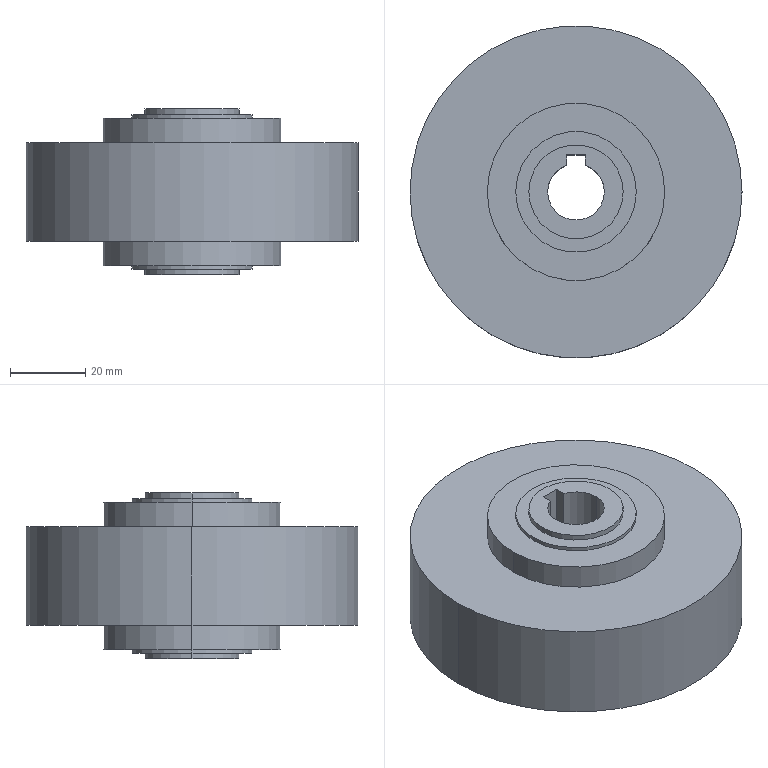Part | STEP file | Mirror ZX3YN | 1 solid | 40 faces | box 88 x 88 x 44 mm | volume 175155 mm3 | cylinder 23 | plane 11 | cone 6 | commonest cylinder face diameters 3.3 x6 25 x4 32 x4 47 x4 15 x3 88 x2
STEP:
#1=CARTESIAN_POINT('',(-35.466,-18.571,-1.5));
#2=VERTEX_POINT('',#1);
#3=CARTESIAN_POINT('',(-33.816,-21.429,-1.5));
#4=VERTEX_POINT('',#3);
#5=CARTESIAN_POINT('',(-34.641,-20.,-1.5));
#6=DIRECTION('',(0.,0.,1.));
#7=DIRECTION('',(-0.5,0.866,0.));
#8=AXIS2_PLACEMENT_3D('',#5,#6,#7);
#9=CIRCLE('',#8,1.65);
#10=EDGE_CURVE('',#2,#4,#9,.T.);
#11=ORIENTED_EDGE('',*,*,#10,.T.);
#12=CARTESIAN_POINT('',(-33.816,-21.429,-13.));
#13=VERTEX_POINT('',#12);
#14=CARTESIAN_POINT('',(-33.816,-21.429,-13.));
#15=DIRECTION('',(0.,0.,-1.));
#16=VECTOR('',#15,1000.);
#17=LINE('',#14,#16);
#18=EDGE_CURVE('',#4,#13,#17,.T.);
#19=ORIENTED_EDGE('',*,*,#18,.T.);
#20=CARTESIAN_POINT('',(-35.466,-18.571,-13.));
#21=VERTEX_POINT('',#20);
#22=CARTESIAN_POINT('',(-34.641,-20.,-13.));
#23=DIRECTION('',(0.,0.,1.));
#24=DIRECTION('',(-0.5,0.866,0.));
#25=AXIS2_PLACEMENT_3D('',#22,#23,#24);
#26=CIRCLE('',#25,1.65);
#27=EDGE_CURVE('',#21,#13,#26,.T.);
#28=ORIENTED_EDGE('',*,*,#27,.F.);
#29=CARTESIAN_POINT('',(-35.466,-18.571,-13.));
#30=DIRECTION('',(0.,0.,-1.));
#31=VECTOR('',#30,1000.);
#32=LINE('',#29,#31);
#33=EDGE_CURVE('',#2,#21,#32,.T.);
#34=ORIENTED_EDGE('',*,*,#33,.F.);
#35=EDGE_LOOP('',(#11,#19,#28,#34));
#36=FACE_OUTER_BOUND('',#35,.T.);
#37=CARTESIAN_POINT('',(-34.641,-20.,-13.));
#38=DIRECTION('',(0.,0.,-1.));
#39=DIRECTION('',(-0.5,0.866,0.));
#40=AXIS2_PLACEMENT_3D('',#37,#38,#39);
#41=CYLINDRICAL_SURFACE('',#40,1.65);
#42=ADVANCED_FACE('',(#36),#41,.F.);
#43=CARTESIAN_POINT('',(-34.641,-20.,-0.5086));
#44=VERTEX_POINT('',#43);
#45=CARTESIAN_POINT('',(-35.466,-18.571,-1.5));
#46=DIRECTION('',(-0.4286,0.7423,-0.515));
#47=VECTOR('',#46,1000.);
#48=LINE('',#45,#47);
#49=EDGE_CURVE('',#44,#2,#48,.T.);
#50=ORIENTED_EDGE('',*,*,#49,.F.);
#51=CARTESIAN_POINT('',(-33.816,-21.429,-1.5));
#52=DIRECTION('',(0.4286,-0.7423,-0.515));
#53=VECTOR('',#52,1000.);
#54=LINE('',#51,#53);
#55=EDGE_CURVE('',#44,#4,#54,.T.);
#56=ORIENTED_EDGE('',*,*,#55,.T.);
#57=ORIENTED_EDGE('',*,*,#10,.F.);
#58=EDGE_LOOP('',(#50,#56,#57));
#59=FACE_OUTER_BOUND('',#58,.T.);
#60=CARTESIAN_POINT('',(-34.641,-20.,-1.5));
#61=DIRECTION('',(0.,0.,-1.));
#62=DIRECTION('',(-0.5,0.866,0.));
#63=AXIS2_PLACEMENT_3D('',#60,#61,#62);
#64=CONICAL_SURFACE('',#63,1.65,1.03);
#65=ADVANCED_FACE('',(#59),#64,.F.);
#66=CARTESIAN_POINT('',(33.816,-21.429,-1.5));
#67=VERTEX_POINT('',#66);
#68=CARTESIAN_POINT('',(35.466,-18.571,-1.5));
#69=VERTEX_POINT('',#68);
#70=CARTESIAN_POINT('',(34.641,-20.,-1.5));
#71=DIRECTION('',(0.,0.,1.));
#72=DIRECTION('',(-0.5,-0.866,0.));
#73=AXIS2_PLACEMENT_3D('',#70,#71,#72);
#74=CIRCLE('',#73,1.65);
#75=EDGE_CURVE('',#67,#69,#74,.T.);
#76=ORIENTED_EDGE('',*,*,#75,.T.);
#77=CARTESIAN_POINT('',(35.466,-18.571,-13.));
#78=VERTEX_POINT('',#77);
#79=CARTESIAN_POINT('',(35.466,-18.571,-13.));
#80=DIRECTION('',(0.,0.,-1.));
#81=VECTOR('',#80,1000.);
#82=LINE('',#79,#81);
#83=EDGE_CURVE('',#69,#78,#82,.T.);
#84=ORIENTED_EDGE('',*,*,#83,.T.);
#85=CARTESIAN_POINT('',(33.816,-21.429,-13.));
#86=VERTEX_POINT('',#85);
#87=CARTESIAN_POINT('',(34.641,-20.,-13.));
#88=DIRECTION('',(0.,0.,1.));
#89=DIRECTION('',(-0.5,-0.866,0.));
#90=AXIS2_PLACEMENT_3D('',#87,#88,#89);
#91=CIRCLE('',#90,1.65);
#92=EDGE_CURVE('',#86,#78,#91,.T.);
#93=ORIENTED_EDGE('',*,*,#92,.F.);
#94=CARTESIAN_POINT('',(33.816,-21.429,-13.));
#95=DIRECTION('',(0.,0.,-1.));
#96=VECTOR('',#95,1000.);
#97=LINE('',#94,#96);
#98=EDGE_CURVE('',#67,#86,#97,.T.);
#99=ORIENTED_EDGE('',*,*,#98,.F.);
#100=EDGE_LOOP('',(#76,#84,#93,#99));
#101=FACE_OUTER_BOUND('',#100,.T.);
#102=CARTESIAN_POINT('',(34.641,-20.,-13.));
#103=DIRECTION('',(0.,0.,-1.));
#104=DIRECTION('',(-0.5,-0.866,0.));
#105=AXIS2_PLACEMENT_3D('',#102,#103,#104);
#106=CYLINDRICAL_SURFACE('',#105,1.65);
#107=ADVANCED_FACE('',(#101),#106,.F.);
#108=CARTESIAN_POINT('',(34.641,-20.,-0.5086));
#109=VERTEX_POINT('',#108);
#110=CARTESIAN_POINT('',(33.816,-21.429,-1.5));
#111=DIRECTION('',(-0.4286,-0.7423,-0.515));
#112=VECTOR('',#111,1000.);
#113=LINE('',#110,#112);
#114=EDGE_CURVE('',#109,#67,#113,.T.);
#115=ORIENTED_EDGE('',*,*,#114,.F.);
#116=CARTESIAN_POINT('',(35.466,-18.571,-1.5));
#117=DIRECTION('',(0.4286,0.7423,-0.515));
#118=VECTOR('',#117,1000.);
#119=LINE('',#116,#118);
#120=EDGE_CURVE('',#109,#69,#119,.T.);
#121=ORIENTED_EDGE('',*,*,#120,.T.);
#122=ORIENTED_EDGE('',*,*,#75,.F.);
#123=EDGE_LOOP('',(#115,#121,#122));
#124=FACE_OUTER_BOUND('',#123,.T.);
#125=CARTESIAN_POINT('',(34.641,-20.,-1.5));
#126=DIRECTION('',(0.,0.,-1.));
#127=DIRECTION('',(-0.5,-0.866,0.));
#128=AXIS2_PLACEMENT_3D('',#125,#126,#127);
#129=CONICAL_SURFACE('',#128,1.65,1.03);
#130=ADVANCED_FACE('',(#124),#129,.F.);
#131=CARTESIAN_POINT('',(1.65,40.,-1.5));
#132=VERTEX_POINT('',#131);
#133=CARTESIAN_POINT('',(-1.65,40.,-1.5));
#134=VERTEX_POINT('',#133);
#135=CARTESIAN_POINT('',(0.,40.,-1.5));
#136=DIRECTION('',(0.,0.,1.));
#137=DIRECTION('',(1.,0.,0.));
#138=AXIS2_PLACEMENT_3D('',#135,#136,#137);
#139=CIRCLE('',#138,1.65);
#140=EDGE_CURVE('',#132,#134,#139,.T.);
#141=ORIENTED_EDGE('',*,*,#140,.T.);
#142=CARTESIAN_POINT('',(-1.65,40.,-13.));
#143=VERTEX_POINT('',#142);
#144=CARTESIAN_POINT('',(-1.65,40.,-13.));
#145=DIRECTION('',(0.,0.,-1.));
#146=VECTOR('',#145,1000.);
#147=LINE('',#144,#146);
#148=EDGE_CURVE('',#134,#143,#147,.T.);
#149=ORIENTED_EDGE('',*,*,#148,.T.);
#150=CARTESIAN_POINT('',(1.65,40.,-13.));
#151=VERTEX_POINT('',#150);
#152=CARTESIAN_POINT('',(0.,40.,-13.));
#153=DIRECTION('',(0.,0.,1.));
#154=DIRECTION('',(1.,0.,0.));
#155=AXIS2_PLACEMENT_3D('',#152,#153,#154);
#156=CIRCLE('',#155,1.65);
#157=EDGE_CURVE('',#151,#143,#156,.T.);
#158=ORIENTED_EDGE('',*,*,#157,.F.);
#159=CARTESIAN_POINT('',(1.65,40.,-13.));
#160=DIRECTION('',(0.,0.,-1.));
#161=VECTOR('',#160,1000.);
#162=LINE('',#159,#161);
#163=EDGE_CURVE('',#132,#151,#162,.T.);
#164=ORIENTED_EDGE('',*,*,#163,.F.);
#165=EDGE_LOOP('',(#141,#149,#158,#164));
#166=FACE_OUTER_BOUND('',#165,.T.);
#167=CARTESIAN_POINT('',(0.,40.,-13.));
#168=DIRECTION('',(0.,0.,-1.));
#169=DIRECTION('',(1.,0.,0.));
#170=AXIS2_PLACEMENT_3D('',#167,#168,#169);
#171=CYLINDRICAL_SURFACE('',#170,1.65);
#172=ADVANCED_FACE('',(#166),#171,.F.);
#173=CARTESIAN_POINT('',(0.,40.,-0.5086));
#174=VERTEX_POINT('',#173);
#175=CARTESIAN_POINT('',(1.65,40.,-1.5));
#176=DIRECTION('',(0.8572,0.,-0.515));
#177=VECTOR('',#176,1000.);
#178=LINE('',#175,#177);
#179=EDGE_CURVE('',#174,#132,#178,.T.);
#180=ORIENTED_EDGE('',*,*,#179,.F.);
#181=CARTESIAN_POINT('',(-1.65,40.,-1.5));
#182=DIRECTION('',(-0.8572,0.,-0.515));
#183=VECTOR('',#182,1000.);
#184=LINE('',#181,#183);
#185=EDGE_CURVE('',#174,#134,#184,.T.);
#186=ORIENTED_EDGE('',*,*,#185,.T.);
#187=ORIENTED_EDGE('',*,*,#140,.F.);
#188=EDGE_LOOP('',(#180,#186,#187));
#189=FACE_OUTER_BOUND('',#188,.T.);
#190=CARTESIAN_POINT('',(0.,40.,-1.5));
#191=DIRECTION('',(0.,0.,-1.));
#192=DIRECTION('',(1.,0.,0.));
#193=AXIS2_PLACEMENT_3D('',#190,#191,#192);
#194=CONICAL_SURFACE('',#193,1.65,1.03);
#195=ADVANCED_FACE('',(#189),#194,.F.);
#196=CARTESIAN_POINT('',(-2.5,7.071,22.));
#197=VERTEX_POINT('',#196);
#198=CARTESIAN_POINT('',(-7.5,0.,22.));
#199=VERTEX_POINT('',#198);
#200=CARTESIAN_POINT('',(0.,0.,22.));
#201=DIRECTION('',(0.,0.,1.));
#202=DIRECTION('',(1.,0.,0.));
#203=AXIS2_PLACEMENT_3D('',#200,#201,#202);
#204=CIRCLE('',#203,7.5);
#205=EDGE_CURVE('',#197,#199,#204,.T.);
#206=ORIENTED_EDGE('',*,*,#205,.T.);
#207=CARTESIAN_POINT('',(-7.5,0.,-22.));
#208=VERTEX_POINT('',#207);
#209=CARTESIAN_POINT('',(-7.5,0.,22.));
#210=DIRECTION('',(0.,0.,-1.));
#211=VECTOR('',#210,1000.);
#212=LINE('',#209,#211);
#213=EDGE_CURVE('',#199,#208,#212,.T.);
#214=ORIENTED_EDGE('',*,*,#213,.T.);
#215=CARTESIAN_POINT('',(-2.5,7.071,-22.));
#216=VERTEX_POINT('',#215);
#217=CARTESIAN_POINT('',(0.,0.,-22.));
#218=DIRECTION('',(0.,0.,1.));
#219=DIRECTION('',(1.,0.,0.));
#220=AXIS2_PLACEMENT_3D('',#217,#218,#219);
#221=CIRCLE('',#220,7.5);
#222=EDGE_CURVE('',#216,#208,#221,.T.);
#223=ORIENTED_EDGE('',*,*,#222,.F.);
#224=CARTESIAN_POINT('',(-2.5,7.071,22.));
#225=DIRECTION('',(0.,0.,-1.));
#226=VECTOR('',#225,1000.);
#227=LINE('',#224,#226);
#228=EDGE_CURVE('',#197,#216,#227,.T.);
#229=ORIENTED_EDGE('',*,*,#228,.F.);
#230=EDGE_LOOP('',(#206,#214,#223,#229));
#231=FACE_OUTER_BOUND('',#230,.T.);
#232=CARTESIAN_POINT('',(0.,0.,22.));
#233=DIRECTION('',(0.,0.,-1.));
#234=DIRECTION('',(1.,0.,0.));
#235=AXIS2_PLACEMENT_3D('',#232,#233,#234);
#236=CYLINDRICAL_SURFACE('',#235,7.5);
#237=ADVANCED_FACE('',(#231),#236,.F.);
#238=ORIENTED_EDGE('',*,*,#213,.F.);
#239=CARTESIAN_POINT('',(7.5,0.,22.));
#240=VERTEX_POINT('',#239);
#241=CARTESIAN_POINT('',(0.,0.,22.));
#242=DIRECTION('',(0.,0.,1.));
#243=DIRECTION('',(1.,0.,0.));
#244=AXIS2_PLACEMENT_3D('',#241,#242,#243);
#245=CIRCLE('',#244,7.5);
#246=EDGE_CURVE('',#199,#240,#245,.T.);
#247=ORIENTED_EDGE('',*,*,#246,.T.);
#248=CARTESIAN_POINT('',(7.5,0.,-22.));
#249=VERTEX_POINT('',#248);
#250=CARTESIAN_POINT('',(7.5,0.,22.));
#251=DIRECTION('',(0.,0.,-1.));
#252=VECTOR('',#251,1000.);
#253=LINE('',#250,#252);
#254=EDGE_CURVE('',#240,#249,#253,.T.);
#255=ORIENTED_EDGE('',*,*,#254,.T.);
#256=CARTESIAN_POINT('',(0.,0.,-22.));
#257=DIRECTION('',(0.,0.,1.));
#258=DIRECTION('',(1.,0.,0.));
#259=AXIS2_PLACEMENT_3D('',#256,#257,#258);
#260=CIRCLE('',#259,7.5);
#261=EDGE_CURVE('',#208,#249,#260,.T.);
#262=ORIENTED_EDGE('',*,*,#261,.F.);
#263=EDGE_LOOP('',(#238,#247,#255,#262));
#264=FACE_OUTER_BOUND('',#263,.T.);
#265=CARTESIAN_POINT('',(0.,0.,22.));
#266=DIRECTION('',(0.,0.,-1.));
#267=DIRECTION('',(1.,0.,0.));
#268=AXIS2_PLACEMENT_3D('',#265,#266,#267);
#269=CYLINDRICAL_SURFACE('',#268,7.5);
#270=ADVANCED_FACE('',(#264),#269,.F.);
#271=CARTESIAN_POINT('',(-12.5,0.,22.));
#272=VERTEX_POINT('',#271);
#273=CARTESIAN_POINT('',(12.5,0.,22.));
#274=VERTEX_POINT('',#273);
#275=CARTESIAN_POINT('',(0.,0.,22.));
#276=DIRECTION('',(0.,0.,1.));
#277=DIRECTION('',(1.,0.,0.));
#278=AXIS2_PLACEMENT_3D('',#275,#276,#277);
#279=CIRCLE('',#278,12.5);
#280=EDGE_CURVE('',#272,#274,#279,.T.);
#281=ORIENTED_EDGE('',*,*,#280,.F.);
#282=CARTESIAN_POINT('',(-12.5,0.,20.5));
#283=VERTEX_POINT('',#282);
#284=CARTESIAN_POINT('',(-12.5,0.,22.));
#285=DIRECTION('',(0.,0.,-1.));
#286=VECTOR('',#285,1000.);
#287=LINE('',#284,#286);
#288=EDGE_CURVE('',#272,#283,#287,.T.);
#289=ORIENTED_EDGE('',*,*,#288,.T.);
#290=CARTESIAN_POINT('',(12.5,0.,20.5));
#291=VERTEX_POINT('',#290);
#292=CARTESIAN_POINT('',(0.,0.,20.5));
#293=DIRECTION('',(0.,0.,-1.));
#294=DIRECTION('',(-1.,0.,0.));
#295=AXIS2_PLACEMENT_3D('',#292,#293,#294);
#296=CIRCLE('',#295,12.5);
#297=EDGE_CURVE('',#291,#283,#296,.T.);
#298=ORIENTED_EDGE('',*,*,#297,.F.);
#299=CARTESIAN_POINT('',(12.5,0.,22.));
#300=DIRECTION('',(0.,0.,-1.));
#301=VECTOR('',#300,1000.);
#302=LINE('',#299,#301);
#303=EDGE_CURVE('',#274,#291,#302,.T.);
#304=ORIENTED_EDGE('',*,*,#303,.F.);
#305=EDGE_LOOP('',(#281,#289,#298,#304));
#306=FACE_OUTER_BOUND('',#305,.T.);
#307=CARTESIAN_POINT('',(0.,0.,22.));
#308=DIRECTION('',(0.,0.,-1.));
#309=DIRECTION('',(1.,0.,0.));
#310=AXIS2_PLACEMENT_3D('',#307,#308,#309);
#311=CYLINDRICAL_SURFACE('',#310,12.5);
#312=ADVANCED_FACE('',(#306),#311,.T.);
#313=CARTESIAN_POINT('',(-16.,0.,20.5));
#314=VERTEX_POINT('',#313);
#315=CARTESIAN_POINT('',(16.,0.,20.5));
#316=VERTEX_POINT('',#315);
#317=CARTESIAN_POINT('',(0.,0.,20.5));
#318=DIRECTION('',(0.,0.,1.));
#319=DIRECTION('',(1.,0.,0.));
#320=AXIS2_PLACEMENT_3D('',#317,#318,#319);
#321=CIRCLE('',#320,16.);
#322=EDGE_CURVE('',#314,#316,#321,.T.);
#323=ORIENTED_EDGE('',*,*,#322,.F.);
#324=CARTESIAN_POINT('',(-16.,0.,19.5));
#325=VERTEX_POINT('',#324);
#326=CARTESIAN_POINT('',(-16.,0.,20.5));
#327=DIRECTION('',(0.,0.,-1.));
#328=VECTOR('',#327,1000.);
#329=LINE('',#326,#328);
#330=EDGE_CURVE('',#314,#325,#329,.T.);
#331=ORIENTED_EDGE('',*,*,#330,.T.);
#332=CARTESIAN_POINT('',(16.,0.,19.5));
#333=VERTEX_POINT('',#332);
#334=CARTESIAN_POINT('',(0.,0.,19.5));
#335=DIRECTION('',(0.,0.,-1.));
#336=DIRECTION('',(-1.,0.,0.));
#337=AXIS2_PLACEMENT_3D('',#334,#335,#336);
#338=CIRCLE('',#337,16.);
#339=EDGE_CURVE('',#333,#325,#338,.T.);
#340=ORIENTED_EDGE('',*,*,#339,.F.);
#341=CARTESIAN_POINT('',(16.,0.,20.5));
#342=DIRECTION('',(0.,0.,-1.));
#343=VECTOR('',#342,1000.);
#344=LINE('',#341,#343);
#345=EDGE_CURVE('',#316,#333,#344,.T.);
#346=ORIENTED_EDGE('',*,*,#345,.F.);
#347=EDGE_LOOP('',(#323,#331,#340,#346));
#348=FACE_OUTER_BOUND('',#347,.T.);
#349=CARTESIAN_POINT('',(0.,0.,20.5));
#350=DIRECTION('',(0.,0.,-1.));
#351=DIRECTION('',(1.,0.,0.));
#352=AXIS2_PLACEMENT_3D('',#349,#350,#351);
#353=CYLINDRICAL_SURFACE('',#352,16.);
#354=ADVANCED_FACE('',(#348),#353,.T.);
#355=CARTESIAN_POINT('',(-23.5,0.,19.5));
#356=VERTEX_POINT('',#355);
#357=CARTESIAN_POINT('',(23.5,0.,19.5));
#358=VERTEX_POINT('',#357);
#359=CARTESIAN_POINT('',(0.,0.,19.5));
#360=DIRECTION('',(0.,0.,1.));
#361=DIRECTION('',(1.,0.,0.));
#362=AXIS2_PLACEMENT_3D('',#359,#360,#361);
#363=CIRCLE('',#362,23.5);
#364=EDGE_CURVE('',#356,#358,#363,.T.);
#365=ORIENTED_EDGE('',*,*,#364,.F.);
#366=CARTESIAN_POINT('',(-23.5,0.,13.));
#367=VERTEX_POINT('',#366);
#368=CARTESIAN_POINT('',(-23.5,0.,19.5));
#369=DIRECTION('',(0.,0.,-1.));
#370=VECTOR('',#369,1000.);
#371=LINE('',#368,#370);
#372=EDGE_CURVE('',#356,#367,#371,.T.);
#373=ORIENTED_EDGE('',*,*,#372,.T.);
#374=CARTESIAN_POINT('',(23.5,0.,13.));
#375=VERTEX_POINT('',#374);
#376=CARTESIAN_POINT('',(0.,0.,13.));
#377=DIRECTION('',(0.,0.,1.));
#378=DIRECTION('',(1.,0.,0.));
#379=AXIS2_PLACEMENT_3D('',#376,#377,#378);
#380=CIRCLE('',#379,23.5);
#381=EDGE_CURVE('',#367,#375,#380,.T.);
#382=ORIENTED_EDGE('',*,*,#381,.T.);
#383=CARTESIAN_POINT('',(23.5,0.,19.5));
#384=DIRECTION('',(0.,0.,-1.));
#385=VECTOR('',#384,1000.);
#386=LINE('',#383,#385);
#387=EDGE_CURVE('',#358,#375,#386,.T.);
#388=ORIENTED_EDGE('',*,*,#387,.F.);
#389=EDGE_LOOP('',(#365,#373,#382,#388));
#390=FACE_OUTER_BOUND('',#389,.T.);
#391=CARTESIAN_POINT('',(0.,0.,19.5));
#392=DIRECTION('',(0.,0.,-1.));
#393=DIRECTION('',(1.,0.,0.));
#394=AXIS2_PLACEMENT_3D('',#391,#392,#393);
#395=CYLINDRICAL_SURFACE('',#394,23.5);
#396=ADVANCED_FACE('',(#390),#395,.T.);
#397=CARTESIAN_POINT('',(-12.5,0.,-22.));
#398=VERTEX_POINT('',#397);
#399=CARTESIAN_POINT('',(12.5,0.,-22.));
#400=VERTEX_POINT('',#399);
#401=CARTESIAN_POINT('',(0.,0.,-22.));
#402=DIRECTION('',(0.,0.,1.));
#403=DIRECTION('',(1.,0.,0.));
#404=AXIS2_PLACEMENT_3D('',#401,#402,#403);
#405=CIRCLE('',#404,12.5);
#406=EDGE_CURVE('',#398,#400,#405,.T.);
#407=ORIENTED_EDGE('',*,*,#406,.T.);
#408=CARTESIAN_POINT('',(12.5,0.,-20.5));
#409=VERTEX_POINT('',#408);
#410=CARTESIAN_POINT('',(12.5,0.,-22.));
#411=DIRECTION('',(0.,0.,1.));
#412=VECTOR('',#411,1000.);
#413=LINE('',#410,#412);
#414=EDGE_CURVE('',#400,#409,#413,.T.);
#415=ORIENTED_EDGE('',*,*,#414,.T.);
#416=CARTESIAN_POINT('',(-12.5,0.,-20.5));
#417=VERTEX_POINT('',#416);
#418=CARTESIAN_POINT('',(0.,0.,-20.5));
#419=DIRECTION('',(0.,0.,1.));
#420=DIRECTION('',(1.,0.,0.));
#421=AXIS2_PLACEMENT_3D('',#418,#419,#420);
#422=CIRCLE('',#421,12.5);
#423=EDGE_CURVE('',#417,#409,#422,.T.);
#424=ORIENTED_EDGE('',*,*,#423,.F.);
#425=CARTESIAN_POINT('',(-12.5,0.,-22.));
#426=DIRECTION('',(0.,0.,1.));
#427=VECTOR('',#426,1000.);
#428=LINE('',#425,#427);
#429=EDGE_CURVE('',#398,#417,#428,.T.);
#430=ORIENTED_EDGE('',*,*,#429,.F.);
#431=EDGE_LOOP('',(#407,#415,#424,#430));
#432=FACE_OUTER_BOUND('',#431,.T.);
#433=CARTESIAN_POINT('',(0.,0.,-22.));
#434=DIRECTION('',(0.,0.,1.));
#435=DIRECTION('',(-1.,0.,0.));
#436=AXIS2_PLACEMENT_3D('',#433,#434,#435);
#437=CYLINDRICAL_SURFACE('',#436,12.5);
#438=ADVANCED_FACE('',(#432),#437,.T.);
#439=CARTESIAN_POINT('',(-16.,0.,-20.5));
#440=VERTEX_POINT('',#439);
#441=CARTESIAN_POINT('',(16.,0.,-20.5));
#442=VERTEX_POINT('',#441);
#443=CARTESIAN_POINT('',(0.,0.,-20.5));
#444=DIRECTION('',(0.,0.,1.));
#445=DIRECTION('',(1.,0.,0.));
#446=AXIS2_PLACEMENT_3D('',#443,#444,#445);
#447=CIRCLE('',#446,16.);
#448=EDGE_CURVE('',#440,#442,#447,.T.);
#449=ORIENTED_EDGE('',*,*,#448,.T.);
#450=CARTESIAN_POINT('',(16.,0.,-19.5));
#451=VERTEX_POINT('',#450);
#452=CARTESIAN_POINT('',(16.,0.,-20.5));
#453=DIRECTION('',(0.,0.,1.));
#454=VECTOR('',#453,1000.);
#455=LINE('',#452,#454);
#456=EDGE_CURVE('',#442,#451,#455,.T.);
#457=ORIENTED_EDGE('',*,*,#456,.T.);
#458=CARTESIAN_POINT('',(-16.,0.,-19.5));
#459=VERTEX_POINT('',#458);
#460=CARTESIAN_POINT('',(0.,0.,-19.5));
#461=DIRECTION('',(0.,0.,1.));
#462=DIRECTION('',(1.,0.,0.));
#463=AXIS2_PLACEMENT_3D('',#460,#461,#462);
#464=CIRCLE('',#463,16.);
#465=EDGE_CURVE('',#459,#451,#464,.T.);
#466=ORIENTED_EDGE('',*,*,#465,.F.);
#467=CARTESIAN_POINT('',(-16.,0.,-20.5));
#468=DIRECTION('',(0.,0.,1.));
#469=VECTOR('',#468,1000.);
#470=LINE('',#467,#469);
#471=EDGE_CURVE('',#440,#459,#470,.T.);
#472=ORIENTED_EDGE('',*,*,#471,.F.);
#473=EDGE_LOOP('',(#449,#457,#466,#472));
#474=FACE_OUTER_BOUND('',#473,.T.);
#475=CARTESIAN_POINT('',(0.,0.,-20.5));
#476=DIRECTION('',(0.,0.,1.));
#477=DIRECTION('',(-1.,0.,0.));
#478=AXIS2_PLACEMENT_3D('',#475,#476,#477);
#479=CYLINDRICAL_SURFACE('',#478,16.);
#480=ADVANCED_FACE('',(#474),#479,.T.);
#481=CARTESIAN_POINT('',(-23.5,0.,-19.5));
#482=VERTEX_POINT('',#481);
#483=CARTESIAN_POINT('',(23.5,0.,-19.5));
#484=VERTEX_POINT('',#483);
#485=CARTESIAN_POINT('',(0.,0.,-19.5));
#486=DIRECTION('',(0.,0.,1.));
#487=DIRECTION('',(1.,0.,0.));
#488=AXIS2_PLACEMENT_3D('',#485,#486,#487);
#489=CIRCLE('',#488,23.5);
#490=EDGE_CURVE('',#482,#484,#489,.T.);
#491=ORIENTED_EDGE('',*,*,#490,.T.);
#492=CARTESIAN_POINT('',(23.5,0.,-13.));
#493=VERTEX_POINT('',#492);
#494=CARTESIAN_POINT('',(23.5,0.,-19.5));
#495=DIRECTION('',(0.,0.,1.));
#496=VECTOR('',#495,1000.);
#497=LINE('',#494,#496);
#498=EDGE_CURVE('',#484,#493,#497,.T.);
#499=ORIENTED_EDGE('',*,*,#498,.T.);
#500=CARTESIAN_POINT('',(-23.5,0.,-13.));
#501=VERTEX_POINT('',#500);
#502=CARTESIAN_POINT('',(0.,0.,-13.));
#503=DIRECTION('',(0.,0.,1.));
#504=DIRECTION('',(1.,0.,0.));
#505=AXIS2_PLACEMENT_3D('',#502,#503,#504);
#506=CIRCLE('',#505,23.5);
#507=EDGE_CURVE('',#501,#493,#506,.T.);
#508=ORIENTED_EDGE('',*,*,#507,.F.);
#509=CARTESIAN_POINT('',(-23.5,0.,-19.5));
#510=DIRECTION('',(0.,0.,1.));
#511=VECTOR('',#510,1000.);
#512=LINE('',#509,#511);
#513=EDGE_CURVE('',#482,#501,#512,.T.);
#514=ORIENTED_EDGE('',*,*,#513,.F.);
#515=EDGE_LOOP('',(#491,#499,#508,#514));
#516=FACE_OUTER_BOUND('',#515,.T.);
#517=CARTESIAN_POINT('',(0.,0.,-19.5));
#518=DIRECTION('',(0.,0.,1.));
#519=DIRECTION('',(-1.,0.,0.));
#520=AXIS2_PLACEMENT_3D('',#517,#518,#519);
#521=CYLINDRICAL_SURFACE('',#520,23.5);
#522=ADVANCED_FACE('',(#516),#521,.T.);
#523=CARTESIAN_POINT('',(-44.,0.,-13.));
#524=VERTEX_POINT('',#523);
#525=CARTESIAN_POINT('',(44.,0.,-13.));
#526=VERTEX_POINT('',#525);
#527=CARTESIAN_POINT('',(0.,0.,-13.));
#528=DIRECTION('',(0.,0.,1.));
#529=DIRECTION('',(1.,0.,0.));
#530=AXIS2_PLACEMENT_3D('',#527,#528,#529);
#531=CIRCLE('',#530,44.);
#532=EDGE_CURVE('',#524,#526,#531,.T.);
#533=ORIENTED_EDGE('',*,*,#532,.T.);
#534=CARTESIAN_POINT('',(44.,0.,13.));
#535=VERTEX_POINT('',#534);
#536=CARTESIAN_POINT('',(44.,0.,-13.));
#537=DIRECTION('',(0.,0.,1.));
#538=VECTOR('',#537,1000.);
#539=LINE('',#536,#538);
#540=EDGE_CURVE('',#526,#535,#539,.T.);
#541=ORIENTED_EDGE('',*,*,#540,.T.);
#542=CARTESIAN_POINT('',(-44.,0.,13.));
#543=VERTEX_POINT('',#542);
#544=CARTESIAN_POINT('',(0.,0.,13.));
#545=DIRECTION('',(0.,0.,1.));
#546=DIRECTION('',(1.,0.,0.));
#547=AXIS2_PLACEMENT_3D('',#544,#545,#546);
#548=CIRCLE('',#547,44.);
#549=EDGE_CURVE('',#543,#535,#548,.T.);
#550=ORIENTED_EDGE('',*,*,#549,.F.);
#551=CARTESIAN_POINT('',(-44.,0.,-13.));
#552=DIRECTION('',(0.,0.,1.));
#553=VECTOR('',#552,1000.);
#554=LINE('',#551,#553);
#555=EDGE_CURVE('',#524,#543,#554,.T.);
#556=ORIENTED_EDGE('',*,*,#555,.F.);
#557=EDGE_LOOP('',(#533,#541,#550,#556));
#558=FACE_OUTER_BOUND('',#557,.T.);
#559=CARTESIAN_POINT('',(0.,0.,-13.));
#560=DIRECTION('',(0.,0.,1.));
#561=DIRECTION('',(-1.,0.,0.));
#562=AXIS2_PLACEMENT_3D('',#559,#560,#561);
#563=CYLINDRICAL_SURFACE('',#562,44.);
#564=ADVANCED_FACE('',(#558),#563,.T.);
#565=ORIENTED_EDGE('',*,*,#448,.F.);
#566=CARTESIAN_POINT('',(0.,0.,-20.5));
#567=DIRECTION('',(0.,0.,1.));
#568=DIRECTION('',(1.,0.,0.));
#569=AXIS2_PLACEMENT_3D('',#566,#567,#568);
#570=CIRCLE('',#569,16.);
#571=EDGE_CURVE('',#442,#440,#570,.T.);
#572=ORIENTED_EDGE('',*,*,#571,.F.);
#573=EDGE_LOOP('',(#565,#572));
#574=FACE_OUTER_BOUND('',#573,.T.);
#575=ORIENTED_EDGE('',*,*,#423,.T.);
#576=CARTESIAN_POINT('',(0.,0.,-20.5));
#577=DIRECTION('',(0.,0.,1.));
#578=DIRECTION('',(1.,0.,0.));
#579=AXIS2_PLACEMENT_3D('',#576,#577,#578);
#580=CIRCLE('',#579,12.5);
#581=EDGE_CURVE('',#409,#417,#580,.T.);
#582=ORIENTED_EDGE('',*,*,#581,.T.);
#583=EDGE_LOOP('',(#575,#582));
#584=FACE_BOUND('',#583,.T.);
#585=CARTESIAN_POINT('',(0.,0.,-20.5));
#586=DIRECTION('',(0.,0.,-1.));
#587=DIRECTION('',(1.,0.,0.));
#588=AXIS2_PLACEMENT_3D('',#585,#586,#587);
#589=PLANE('',#588);
#590=ADVANCED_FACE('',(#574,#584),#589,.T.);
#591=ORIENTED_EDGE('',*,*,#490,.F.);
#592=CARTESIAN_POINT('',(0.,0.,-19.5));
#593=DIRECTION('',(0.,0.,1.));
#594=DIRECTION('',(1.,0.,0.));
#595=AXIS2_PLACEMENT_3D('',#592,#593,#594);
#596=CIRCLE('',#595,23.5);
#597=EDGE_CURVE('',#484,#482,#596,.T.);
#598=ORIENTED_EDGE('',*,*,#597,.F.);
#599=EDGE_LOOP('',(#591,#598));
#600=FACE_OUTER_BOUND('',#599,.T.);
#601=ORIENTED_EDGE('',*,*,#465,.T.);
#602=CARTESIAN_POINT('',(0.,0.,-19.5));
#603=DIRECTION('',(0.,0.,1.));
#604=DIRECTION('',(1.,0.,0.));
#605=AXIS2_PLACEMENT_3D('',#602,#603,#604);
#606=CIRCLE('',#605,16.);
#607=EDGE_CURVE('',#451,#459,#606,.T.);
#608=ORIENTED_EDGE('',*,*,#607,.T.);
#609=EDGE_LOOP('',(#601,#608));
#610=FACE_BOUND('',#609,.T.);
#611=CARTESIAN_POINT('',(0.,0.,-19.5));
#612=DIRECTION('',(0.,0.,-1.));
#613=DIRECTION('',(1.,0.,0.));
#614=AXIS2_PLACEMENT_3D('',#611,#612,#613);
#615=PLANE('',#614);
#616=ADVANCED_FACE('',(#600,#610),#615,.T.);
#617=ORIENTED_EDGE('',*,*,#27,.T.);
#618=CARTESIAN_POINT('',(-34.641,-20.,-13.));
#619=DIRECTION('',(0.,0.,1.));
#620=DIRECTION('',(-0.5,0.866,0.));
#621=AXIS2_PLACEMENT_3D('',#618,#619,#620);
#622=CIRCLE('',#621,1.65);
#623=EDGE_CURVE('',#13,#21,#622,.T.);
#624=ORIENTED_EDGE('',*,*,#623,.T.);
#625=EDGE_LOOP('',(#617,#624));
#626=FACE_BOUND('',#625,.T.);
#627=ORIENTED_EDGE('',*,*,#92,.T.);
#628=CARTESIAN_POINT('',(34.641,-20.,-13.));
#629=DIRECTION('',(0.,0.,1.));
#630=DIRECTION('',(-0.5,-0.866,0.));
#631=AXIS2_PLACEMENT_3D('',#628,#629,#630);
#632=CIRCLE('',#631,1.65);
#633=EDGE_CURVE('',#78,#86,#632,.T.);
#634=ORIENTED_EDGE('',*,*,#633,.T.);
#635=EDGE_LOOP('',(#627,#634));
#636=FACE_BOUND('',#635,.T.);
#637=ORIENTED_EDGE('',*,*,#157,.T.);
#638=CARTESIAN_POINT('',(0.,40.,-13.));
#639=DIRECTION('',(0.,0.,1.));
#640=DIRECTION('',(1.,0.,0.));
#641=AXIS2_PLACEMENT_3D('',#638,#639,#640);
#642=CIRCLE('',#641,1.65);
#643=EDGE_CURVE('',#143,#151,#642,.T.);
#644=ORIENTED_EDGE('',*,*,#643,.T.);
#645=EDGE_LOOP('',(#637,#644));
#646=FACE_BOUND('',#645,.T.);
#647=ORIENTED_EDGE('',*,*,#532,.F.);
#648=CARTESIAN_POINT('',(0.,0.,-13.));
#649=DIRECTION('',(0.,0.,1.));
#650=DIRECTION('',(1.,0.,0.));
#651=AXIS2_PLACEMENT_3D('',#648,#649,#650);
#652=CIRCLE('',#651,44.);
#653=EDGE_CURVE('',#526,#524,#652,.T.);
#654=ORIENTED_EDGE('',*,*,#653,.F.);
#655=EDGE_LOOP('',(#647,#654));
#656=FACE_OUTER_BOUND('',#655,.T.);
#657=ORIENTED_EDGE('',*,*,#507,.T.);
#658=CARTESIAN_POINT('',(0.,0.,-13.));
#659=DIRECTION('',(0.,0.,1.));
#660=DIRECTION('',(1.,0.,0.));
#661=AXIS2_PLACEMENT_3D('',#658,#659,#660);
#662=CIRCLE('',#661,23.5);
#663=EDGE_CURVE('',#493,#501,#662,.T.);
#664=ORIENTED_EDGE('',*,*,#663,.T.);
#665=EDGE_LOOP('',(#657,#664));
#666=FACE_BOUND('',#665,.T.);
#667=CARTESIAN_POINT('',(0.,0.,-13.));
#668=DIRECTION('',(0.,0.,-1.));
#669=DIRECTION('',(1.,0.,0.));
#670=AXIS2_PLACEMENT_3D('',#667,#668,#669);
#671=PLANE('',#670);
#672=ADVANCED_FACE('',(#626,#636,#646,#656,#666),#671,.T.);
#673=ORIENTED_EDGE('',*,*,#540,.F.);
#674=ORIENTED_EDGE('',*,*,#653,.T.);
#675=ORIENTED_EDGE('',*,*,#555,.T.);
#676=CARTESIAN_POINT('',(0.,0.,13.));
#677=DIRECTION('',(0.,0.,1.));
#678=DIRECTION('',(1.,0.,0.));
#679=AXIS2_PLACEMENT_3D('',#676,#677,#678);
#680=CIRCLE('',#679,44.);
#681=EDGE_CURVE('',#535,#543,#680,.T.);
#682=ORIENTED_EDGE('',*,*,#681,.F.);
#683=EDGE_LOOP('',(#673,#674,#675,#682));
#684=FACE_OUTER_BOUND('',#683,.T.);
#685=CARTESIAN_POINT('',(0.,0.,-13.));
#686=DIRECTION('',(0.,0.,1.));
#687=DIRECTION('',(-1.,0.,0.));
#688=AXIS2_PLACEMENT_3D('',#685,#686,#687);
#689=CYLINDRICAL_SURFACE('',#688,44.);
#690=ADVANCED_FACE('',(#684),#689,.T.);
#691=CARTESIAN_POINT('',(0.,0.,13.));
#692=DIRECTION('',(0.,0.,1.));
#693=DIRECTION('',(1.,0.,0.));
#694=AXIS2_PLACEMENT_3D('',#691,#692,#693);
#695=CIRCLE('',#694,23.5);
#696=EDGE_CURVE('',#375,#367,#695,.T.);
#697=ORIENTED_EDGE('',*,*,#696,.F.);
#698=ORIENTED_EDGE('',*,*,#381,.F.);
#699=EDGE_LOOP('',(#697,#698));
#700=FACE_BOUND('',#699,.T.);
#701=ORIENTED_EDGE('',*,*,#549,.T.);
#702=ORIENTED_EDGE('',*,*,#681,.T.);
#703=EDGE_LOOP('',(#701,#702));
#704=FACE_OUTER_BOUND('',#703,.T.);
#705=CARTESIAN_POINT('',(0.,0.,13.));
#706=DIRECTION('',(0.,0.,-1.));
#707=DIRECTION('',(1.,0.,0.));
#708=AXIS2_PLACEMENT_3D('',#705,#706,#707);
#709=PLANE('',#708);
#710=ADVANCED_FACE('',(#700,#704),#709,.F.);
#711=ORIENTED_EDGE('',*,*,#498,.F.);
#712=ORIENTED_EDGE('',*,*,#597,.T.);
#713=ORIENTED_EDGE('',*,*,#513,.T.);
#714=ORIENTED_EDGE('',*,*,#663,.F.);
#715=EDGE_LOOP('',(#711,#712,#713,#714));
#716=FACE_OUTER_BOUND('',#715,.T.);
#717=CARTESIAN_POINT('',(0.,0.,-19.5));
#718=DIRECTION('',(0.,0.,1.));
#719=DIRECTION('',(-1.,0.,0.));
#720=AXIS2_PLACEMENT_3D('',#717,#718,#719);
#721=CYLINDRICAL_SURFACE('',#720,23.5);
#722=ADVANCED_FACE('',(#716),#721,.T.);
#723=ORIENTED_EDGE('',*,*,#456,.F.);
#724=ORIENTED_EDGE('',*,*,#571,.T.);
#725=ORIENTED_EDGE('',*,*,#471,.T.);
#726=ORIENTED_EDGE('',*,*,#607,.F.);
#727=EDGE_LOOP('',(#723,#724,#725,#726));
#728=FACE_OUTER_BOUND('',#727,.T.);
#729=CARTESIAN_POINT('',(0.,0.,-20.5));
#730=DIRECTION('',(0.,0.,1.));
#731=DIRECTION('',(-1.,0.,0.));
#732=AXIS2_PLACEMENT_3D('',#729,#730,#731);
#733=CYLINDRICAL_SURFACE('',#732,16.);
#734=ADVANCED_FACE('',(#728),#733,.T.);
#735=ORIENTED_EDGE('',*,*,#414,.F.);
#736=CARTESIAN_POINT('',(0.,0.,-22.));
#737=DIRECTION('',(0.,0.,1.));
#738=DIRECTION('',(1.,0.,0.));
#739=AXIS2_PLACEMENT_3D('',#736,#737,#738);
#740=CIRCLE('',#739,12.5);
#741=EDGE_CURVE('',#400,#398,#740,.T.);
#742=ORIENTED_EDGE('',*,*,#741,.T.);
#743=ORIENTED_EDGE('',*,*,#429,.T.);
#744=ORIENTED_EDGE('',*,*,#581,.F.);
#745=EDGE_LOOP('',(#735,#742,#743,#744));
#746=FACE_OUTER_BOUND('',#745,.T.);
#747=CARTESIAN_POINT('',(0.,0.,-22.));
#748=DIRECTION('',(0.,0.,1.));
#749=DIRECTION('',(-1.,0.,0.));
#750=AXIS2_PLACEMENT_3D('',#747,#748,#749);
#751=CYLINDRICAL_SURFACE('',#750,12.5);
#752=ADVANCED_FACE('',(#746),#751,.T.);
#753=ORIENTED_EDGE('',*,*,#222,.T.);
#754=ORIENTED_EDGE('',*,*,#261,.T.);
#755=CARTESIAN_POINT('',(2.5,7.071,-22.));
#756=VERTEX_POINT('',#755);
#757=CARTESIAN_POINT('',(0.,0.,-22.));
#758=DIRECTION('',(0.,0.,1.));
#759=DIRECTION('',(1.,0.,0.));
#760=AXIS2_PLACEMENT_3D('',#757,#758,#759);
#761=CIRCLE('',#760,7.5);
#762=EDGE_CURVE('',#249,#756,#761,.T.);
#763=ORIENTED_EDGE('',*,*,#762,.T.);
#764=CARTESIAN_POINT('',(2.5,9.8,-22.));
#765=VERTEX_POINT('',#764);
#766=CARTESIAN_POINT('',(2.5,7.071,-22.));
#767=DIRECTION('',(0.,1.,0.));
#768=VECTOR('',#767,1000.);
#769=LINE('',#766,#768);
#770=EDGE_CURVE('',#756,#765,#769,.T.);
#771=ORIENTED_EDGE('',*,*,#770,.T.);
#772=CARTESIAN_POINT('',(-2.5,9.8,-22.));
#773=VERTEX_POINT('',#772);
#774=CARTESIAN_POINT('',(-2.5,9.8,-22.));
#775=DIRECTION('',(-1.,0.,0.));
#776=VECTOR('',#775,1000.);
#777=LINE('',#774,#776);
#778=EDGE_CURVE('',#765,#773,#777,.T.);
#779=ORIENTED_EDGE('',*,*,#778,.T.);
#780=CARTESIAN_POINT('',(-2.5,7.071,-22.));
#781=DIRECTION('',(0.,-1.,0.));
#782=VECTOR('',#781,1000.);
#783=LINE('',#780,#782);
#784=EDGE_CURVE('',#773,#216,#783,.T.);
#785=ORIENTED_EDGE('',*,*,#784,.T.);
#786=EDGE_LOOP('',(#753,#754,#763,#771,#779,#785));
#787=FACE_BOUND('',#786,.T.);
#788=ORIENTED_EDGE('',*,*,#406,.F.);
#789=ORIENTED_EDGE('',*,*,#741,.F.);
#790=EDGE_LOOP('',(#788,#789));
#791=FACE_OUTER_BOUND('',#790,.T.);
#792=CARTESIAN_POINT('',(0.,0.,-22.));
#793=DIRECTION('',(0.,0.,-1.));
#794=DIRECTION('',(1.,0.,0.));
#795=AXIS2_PLACEMENT_3D('',#792,#793,#794);
#796=PLANE('',#795);
#797=ADVANCED_FACE('',(#787,#791),#796,.T.);
#798=ORIENTED_EDGE('',*,*,#372,.F.);
#799=CARTESIAN_POINT('',(0.,0.,19.5));
#800=DIRECTION('',(0.,0.,1.));
#801=DIRECTION('',(1.,0.,0.));
#802=AXIS2_PLACEMENT_3D('',#799,#800,#801);
#803=CIRCLE('',#802,23.5);
#804=EDGE_CURVE('',#358,#356,#803,.T.);
#805=ORIENTED_EDGE('',*,*,#804,.F.);
#806=ORIENTED_EDGE('',*,*,#387,.T.);
#807=ORIENTED_EDGE('',*,*,#696,.T.);
#808=EDGE_LOOP('',(#798,#805,#806,#807));
#809=FACE_OUTER_BOUND('',#808,.T.);
#810=CARTESIAN_POINT('',(0.,0.,19.5));
#811=DIRECTION('',(0.,0.,-1.));
#812=DIRECTION('',(1.,0.,0.));
#813=AXIS2_PLACEMENT_3D('',#810,#811,#812);
#814=CYLINDRICAL_SURFACE('',#813,23.5);
#815=ADVANCED_FACE('',(#809),#814,.T.);
#816=ORIENTED_EDGE('',*,*,#339,.T.);
#817=CARTESIAN_POINT('',(0.,0.,19.5));
#818=DIRECTION('',(0.,0.,-1.));
#819=DIRECTION('',(-1.,0.,0.));
#820=AXIS2_PLACEMENT_3D('',#817,#818,#819);
#821=CIRCLE('',#820,16.);
#822=EDGE_CURVE('',#325,#333,#821,.T.);
#823=ORIENTED_EDGE('',*,*,#822,.T.);
#824=EDGE_LOOP('',(#816,#823));
#825=FACE_BOUND('',#824,.T.);
#826=ORIENTED_EDGE('',*,*,#804,.T.);
#827=ORIENTED_EDGE('',*,*,#364,.T.);
#828=EDGE_LOOP('',(#826,#827));
#829=FACE_OUTER_BOUND('',#828,.T.);
#830=CARTESIAN_POINT('',(0.,0.,19.5));
#831=DIRECTION('',(0.,0.,1.));
#832=DIRECTION('',(1.,0.,0.));
#833=AXIS2_PLACEMENT_3D('',#830,#831,#832);
#834=PLANE('',#833);
#835=ADVANCED_FACE('',(#825,#829),#834,.T.);
#836=ORIENTED_EDGE('',*,*,#330,.F.);
#837=CARTESIAN_POINT('',(0.,0.,20.5));
#838=DIRECTION('',(0.,0.,1.));
#839=DIRECTION('',(1.,0.,0.));
#840=AXIS2_PLACEMENT_3D('',#837,#838,#839);
#841=CIRCLE('',#840,16.);
#842=EDGE_CURVE('',#316,#314,#841,.T.);
#843=ORIENTED_EDGE('',*,*,#842,.F.);
#844=ORIENTED_EDGE('',*,*,#345,.T.);
#845=ORIENTED_EDGE('',*,*,#822,.F.);
#846=EDGE_LOOP('',(#836,#843,#844,#845));
#847=FACE_OUTER_BOUND('',#846,.T.);
#848=CARTESIAN_POINT('',(0.,0.,20.5));
#849=DIRECTION('',(0.,0.,-1.));
#850=DIRECTION('',(1.,0.,0.));
#851=AXIS2_PLACEMENT_3D('',#848,#849,#850);
#852=CYLINDRICAL_SURFACE('',#851,16.);
#853=ADVANCED_FACE('',(#847),#852,.T.);
#854=ORIENTED_EDGE('',*,*,#297,.T.);
#855=CARTESIAN_POINT('',(0.,0.,20.5));
#856=DIRECTION('',(0.,0.,-1.));
#857=DIRECTION('',(-1.,0.,0.));
#858=AXIS2_PLACEMENT_3D('',#855,#856,#857);
#859=CIRCLE('',#858,12.5);
#860=EDGE_CURVE('',#283,#291,#859,.T.);
#861=ORIENTED_EDGE('',*,*,#860,.T.);
#862=EDGE_LOOP('',(#854,#861));
#863=FACE_BOUND('',#862,.T.);
#864=ORIENTED_EDGE('',*,*,#842,.T.);
#865=ORIENTED_EDGE('',*,*,#322,.T.);
#866=EDGE_LOOP('',(#864,#865));
#867=FACE_OUTER_BOUND('',#866,.T.);
#868=CARTESIAN_POINT('',(0.,0.,20.5));
#869=DIRECTION('',(0.,0.,1.));
#870=DIRECTION('',(1.,0.,0.));
#871=AXIS2_PLACEMENT_3D('',#868,#869,#870);
#872=PLANE('',#871);
#873=ADVANCED_FACE('',(#863,#867),#872,.T.);
#874=ORIENTED_EDGE('',*,*,#288,.F.);
#875=CARTESIAN_POINT('',(0.,0.,22.));
#876=DIRECTION('',(0.,0.,1.));
#877=DIRECTION('',(1.,0.,0.));
#878=AXIS2_PLACEMENT_3D('',#875,#876,#877);
#879=CIRCLE('',#878,12.5);
#880=EDGE_CURVE('',#274,#272,#879,.T.);
#881=ORIENTED_EDGE('',*,*,#880,.F.);
#882=ORIENTED_EDGE('',*,*,#303,.T.);
#883=ORIENTED_EDGE('',*,*,#860,.F.);
#884=EDGE_LOOP('',(#874,#881,#882,#883));
#885=FACE_OUTER_BOUND('',#884,.T.);
#886=CARTESIAN_POINT('',(0.,0.,22.));
#887=DIRECTION('',(0.,0.,-1.));
#888=DIRECTION('',(1.,0.,0.));
#889=AXIS2_PLACEMENT_3D('',#886,#887,#888);
#890=CYLINDRICAL_SURFACE('',#889,12.5);
#891=ADVANCED_FACE('',(#885),#890,.T.);
#892=ORIENTED_EDGE('',*,*,#205,.F.);
#893=CARTESIAN_POINT('',(-2.5,9.8,22.));
#894=VERTEX_POINT('',#893);
#895=CARTESIAN_POINT('',(-2.5,7.071,22.));
#896=DIRECTION('',(0.,-1.,0.));
#897=VECTOR('',#896,1000.);
#898=LINE('',#895,#897);
#899=EDGE_CURVE('',#894,#197,#898,.T.);
#900=ORIENTED_EDGE('',*,*,#899,.F.);
#901=CARTESIAN_POINT('',(2.5,9.8,22.));
#902=VERTEX_POINT('',#901);
#903=CARTESIAN_POINT('',(-2.5,9.8,22.));
#904=DIRECTION('',(-1.,0.,0.));
#905=VECTOR('',#904,1000.);
#906=LINE('',#903,#905);
#907=EDGE_CURVE('',#902,#894,#906,.T.);
#908=ORIENTED_EDGE('',*,*,#907,.F.);
#909=CARTESIAN_POINT('',(2.5,7.071,22.));
#910=VERTEX_POINT('',#909);
#911=CARTESIAN_POINT('',(2.5,7.071,22.));
#912=DIRECTION('',(0.,1.,0.));
#913=VECTOR('',#912,1000.);
#914=LINE('',#911,#913);
#915=EDGE_CURVE('',#910,#902,#914,.T.);
#916=ORIENTED_EDGE('',*,*,#915,.F.);
#917=CARTESIAN_POINT('',(0.,0.,22.));
#918=DIRECTION('',(0.,0.,1.));
#919=DIRECTION('',(1.,0.,0.));
#920=AXIS2_PLACEMENT_3D('',#917,#918,#919);
#921=CIRCLE('',#920,7.5);
#922=EDGE_CURVE('',#240,#910,#921,.T.);
#923=ORIENTED_EDGE('',*,*,#922,.F.);
#924=ORIENTED_EDGE('',*,*,#246,.F.);
#925=EDGE_LOOP('',(#892,#900,#908,#916,#923,#924));
#926=FACE_BOUND('',#925,.T.);
#927=ORIENTED_EDGE('',*,*,#880,.T.);
#928=ORIENTED_EDGE('',*,*,#280,.T.);
#929=EDGE_LOOP('',(#927,#928));
#930=FACE_OUTER_BOUND('',#929,.T.);
#931=CARTESIAN_POINT('',(0.,0.,22.));
#932=DIRECTION('',(0.,0.,1.));
#933=DIRECTION('',(1.,0.,0.));
#934=AXIS2_PLACEMENT_3D('',#931,#932,#933);
#935=PLANE('',#934);
#936=ADVANCED_FACE('',(#926,#930),#935,.T.);
#937=ORIENTED_EDGE('',*,*,#254,.F.);
#938=ORIENTED_EDGE('',*,*,#922,.T.);
#939=CARTESIAN_POINT('',(2.5,7.071,22.));
#940=DIRECTION('',(0.,0.,-1.));
#941=VECTOR('',#940,1000.);
#942=LINE('',#939,#941);
#943=EDGE_CURVE('',#910,#756,#942,.T.);
#944=ORIENTED_EDGE('',*,*,#943,.T.);
#945=ORIENTED_EDGE('',*,*,#762,.F.);
#946=EDGE_LOOP('',(#937,#938,#944,#945));
#947=FACE_OUTER_BOUND('',#946,.T.);
#948=CARTESIAN_POINT('',(0.,0.,22.));
#949=DIRECTION('',(0.,0.,-1.));
#950=DIRECTION('',(1.,0.,0.));
#951=AXIS2_PLACEMENT_3D('',#948,#949,#950);
#952=CYLINDRICAL_SURFACE('',#951,7.5);
#953=ADVANCED_FACE('',(#947),#952,.F.);
#954=ORIENTED_EDGE('',*,*,#784,.F.);
#955=CARTESIAN_POINT('',(-2.5,9.8,22.));
#956=DIRECTION('',(0.,0.,-1.));
#957=VECTOR('',#956,1000.);
#958=LINE('',#955,#957);
#959=EDGE_CURVE('',#894,#773,#958,.T.);
#960=ORIENTED_EDGE('',*,*,#959,.F.);
#961=ORIENTED_EDGE('',*,*,#899,.T.);
#962=ORIENTED_EDGE('',*,*,#228,.T.);
#963=EDGE_LOOP('',(#954,#960,#961,#962));
#964=FACE_OUTER_BOUND('',#963,.T.);
#965=CARTESIAN_POINT('',(-2.5,7.071,22.));
#966=DIRECTION('',(-1.,0.,0.));
#967=DIRECTION('',(0.,0.,-1.));
#968=AXIS2_PLACEMENT_3D('',#965,#966,#967);
#969=PLANE('',#968);
#970=ADVANCED_FACE('',(#964),#969,.F.);
#971=ORIENTED_EDGE('',*,*,#778,.F.);
#972=CARTESIAN_POINT('',(2.5,9.8,22.));
#973=DIRECTION('',(0.,0.,-1.));
#974=VECTOR('',#973,1000.);
#975=LINE('',#972,#974);
#976=EDGE_CURVE('',#902,#765,#975,.T.);
#977=ORIENTED_EDGE('',*,*,#976,.F.);
#978=ORIENTED_EDGE('',*,*,#907,.T.);
#979=ORIENTED_EDGE('',*,*,#959,.T.);
#980=EDGE_LOOP('',(#971,#977,#978,#979));
#981=FACE_OUTER_BOUND('',#980,.T.);
#982=CARTESIAN_POINT('',(-2.5,9.8,22.));
#983=DIRECTION('',(0.,1.,0.));
#984=DIRECTION('',(0.,0.,-1.));
#985=AXIS2_PLACEMENT_3D('',#982,#983,#984);
#986=PLANE('',#985);
#987=ADVANCED_FACE('',(#981),#986,.F.);
#988=ORIENTED_EDGE('',*,*,#770,.F.);
#989=ORIENTED_EDGE('',*,*,#943,.F.);
#990=ORIENTED_EDGE('',*,*,#915,.T.);
#991=ORIENTED_EDGE('',*,*,#976,.T.);
#992=EDGE_LOOP('',(#988,#989,#990,#991));
#993=FACE_OUTER_BOUND('',#992,.T.);
#994=CARTESIAN_POINT('',(2.5,7.071,22.));
#995=DIRECTION('',(1.,0.,0.));
#996=DIRECTION('',(0.,0.,1.));
#997=AXIS2_PLACEMENT_3D('',#994,#995,#996);
#998=PLANE('',#997);
#999=ADVANCED_FACE('',(#993),#998,.F.);
#1000=ORIENTED_EDGE('',*,*,#185,.F.);
#1001=ORIENTED_EDGE('',*,*,#179,.T.);
#1002=CARTESIAN_POINT('',(0.,40.,-1.5));
#1003=DIRECTION('',(0.,0.,1.));
#1004=DIRECTION('',(1.,0.,0.));
#1005=AXIS2_PLACEMENT_3D('',#1002,#1003,#1004);
#1006=CIRCLE('',#1005,1.65);
#1007=EDGE_CURVE('',#134,#132,#1006,.T.);
#1008=ORIENTED_EDGE('',*,*,#1007,.F.);
#1009=EDGE_LOOP('',(#1000,#1001,#1008));
#1010=FACE_OUTER_BOUND('',#1009,.T.);
#1011=CARTESIAN_POINT('',(0.,40.,-1.5));
#1012=DIRECTION('',(0.,0.,-1.));
#1013=DIRECTION('',(1.,0.,0.));
#1014=AXIS2_PLACEMENT_3D('',#1011,#1012,#1013);
#1015=CONICAL_SURFACE('',#1014,1.65,1.03);
#1016=ADVANCED_FACE('',(#1010),#1015,.F.);
#1017=ORIENTED_EDGE('',*,*,#148,.F.);
#1018=ORIENTED_EDGE('',*,*,#1007,.T.);
#1019=ORIENTED_EDGE('',*,*,#163,.T.);
#1020=ORIENTED_EDGE('',*,*,#643,.F.);
#1021=EDGE_LOOP('',(#1017,#1018,#1019,#1020));
#1022=FACE_OUTER_BOUND('',#1021,.T.);
#1023=CARTESIAN_POINT('',(0.,40.,-13.));
#1024=DIRECTION('',(0.,0.,-1.));
#1025=DIRECTION('',(1.,0.,0.));
#1026=AXIS2_PLACEMENT_3D('',#1023,#1024,#1025);
#1027=CYLINDRICAL_SURFACE('',#1026,1.65);
#1028=ADVANCED_FACE('',(#1022),#1027,.F.);
#1029=ORIENTED_EDGE('',*,*,#120,.F.);
#1030=ORIENTED_EDGE('',*,*,#114,.T.);
#1031=CARTESIAN_POINT('',(34.641,-20.,-1.5));
#1032=DIRECTION('',(0.,0.,1.));
#1033=DIRECTION('',(-0.5,-0.866,0.));
#1034=AXIS2_PLACEMENT_3D('',#1031,#1032,#1033);
#1035=CIRCLE('',#1034,1.65);
#1036=EDGE_CURVE('',#69,#67,#1035,.T.);
#1037=ORIENTED_EDGE('',*,*,#1036,.F.);
#1038=EDGE_LOOP('',(#1029,#1030,#1037));
#1039=FACE_OUTER_BOUND('',#1038,.T.);
#1040=CARTESIAN_POINT('',(34.641,-20.,-1.5));
#1041=DIRECTION('',(0.,0.,-1.));
#1042=DIRECTION('',(-0.5,-0.866,0.));
#1043=AXIS2_PLACEMENT_3D('',#1040,#1041,#1042);
#1044=CONICAL_SURFACE('',#1043,1.65,1.03);
#1045=ADVANCED_FACE('',(#1039),#1044,.F.);
#1046=ORIENTED_EDGE('',*,*,#83,.F.);
#1047=ORIENTED_EDGE('',*,*,#1036,.T.);
#1048=ORIENTED_EDGE('',*,*,#98,.T.);
#1049=ORIENTED_EDGE('',*,*,#633,.F.);
#1050=EDGE_LOOP('',(#1046,#1047,#1048,#1049));
#1051=FACE_OUTER_BOUND('',#1050,.T.);
#1052=CARTESIAN_POINT('',(34.641,-20.,-13.));
#1053=DIRECTION('',(0.,0.,-1.));
#1054=DIRECTION('',(-0.5,-0.866,0.));
#1055=AXIS2_PLACEMENT_3D('',#1052,#1053,#1054);
#1056=CYLINDRICAL_SURFACE('',#1055,1.65);
#1057=ADVANCED_FACE('',(#1051),#1056,.F.);
#1058=ORIENTED_EDGE('',*,*,#55,.F.);
#1059=ORIENTED_EDGE('',*,*,#49,.T.);
#1060=CARTESIAN_POINT('',(-34.641,-20.,-1.5));
#1061=DIRECTION('',(0.,0.,1.));
#1062=DIRECTION('',(-0.5,0.866,0.));
#1063=AXIS2_PLACEMENT_3D('',#1060,#1061,#1062);
#1064=CIRCLE('',#1063,1.65);
#1065=EDGE_CURVE('',#4,#2,#1064,.T.);
#1066=ORIENTED_EDGE('',*,*,#1065,.F.);
#1067=EDGE_LOOP('',(#1058,#1059,#1066));
#1068=FACE_OUTER_BOUND('',#1067,.T.);
#1069=CARTESIAN_POINT('',(-34.641,-20.,-1.5));
#1070=DIRECTION('',(0.,0.,-1.));
#1071=DIRECTION('',(-0.5,0.866,0.));
#1072=AXIS2_PLACEMENT_3D('',#1069,#1070,#1071);
#1073=CONICAL_SURFACE('',#1072,1.65,1.03);
#1074=ADVANCED_FACE('',(#1068),#1073,.F.);
#1075=ORIENTED_EDGE('',*,*,#18,.F.);
#1076=ORIENTED_EDGE('',*,*,#1065,.T.);
#1077=ORIENTED_EDGE('',*,*,#33,.T.);
#1078=ORIENTED_EDGE('',*,*,#623,.F.);
#1079=EDGE_LOOP('',(#1075,#1076,#1077,#1078));
#1080=FACE_OUTER_BOUND('',#1079,.T.);
#1081=CARTESIAN_POINT('',(-34.641,-20.,-13.));
#1082=DIRECTION('',(0.,0.,-1.));
#1083=DIRECTION('',(-0.5,0.866,0.));
#1084=AXIS2_PLACEMENT_3D('',#1081,#1082,#1083);
#1085=CYLINDRICAL_SURFACE('',#1084,1.65);
#1086=ADVANCED_FACE('',(#1080),#1085,.F.);
#1087=CLOSED_SHELL('',(#42,#65,#107,#130,#172,#195,#237,#270,#312,#354,#396,#438,#480,#522,#564,#590,#616,#672,#690,#710,#722,#734,#752,#797,#815,#835,#853,#873,#891,#936,#953,#970,#987,#999,#1016,#1028,#1045,#1057,#1074,#1086));
#1088=MANIFOLD_SOLID_BREP('',#1087);
#1089=CARTESIAN_POINT('',(0.,0.,0.));
#1090=DIRECTION('',(0.,0.,1.));
#1091=DIRECTION('',(1.,0.,0.));
#1092=AXIS2_PLACEMENT_3D('',#1089,#1090,#1091);
#1093=(LENGTH_UNIT()NAMED_UNIT(*)SI_UNIT(.MILLI.,.METRE.));
#1094=UNCERTAINTY_MEASURE_WITH_UNIT(LENGTH_MEASURE(0.00001),#1093,'','');
#1095=(NAMED_UNIT(*)PLANE_ANGLE_UNIT()SI_UNIT($,.RADIAN.));
#1096=(NAMED_UNIT(*)SI_UNIT($,.STERADIAN.)SOLID_ANGLE_UNIT());
#1097=(GEOMETRIC_REPRESENTATION_CONTEXT(3)GLOBAL_UNCERTAINTY_ASSIGNED_CONTEXT((#1094))GLOBAL_UNIT_ASSIGNED_CONTEXT((#1093,#1095,#1096))REPRESENTATION_CONTEXT('',''));
#1098=ADVANCED_BREP_SHAPE_REPRESENTATION('',(#1088,#1092),#1097);